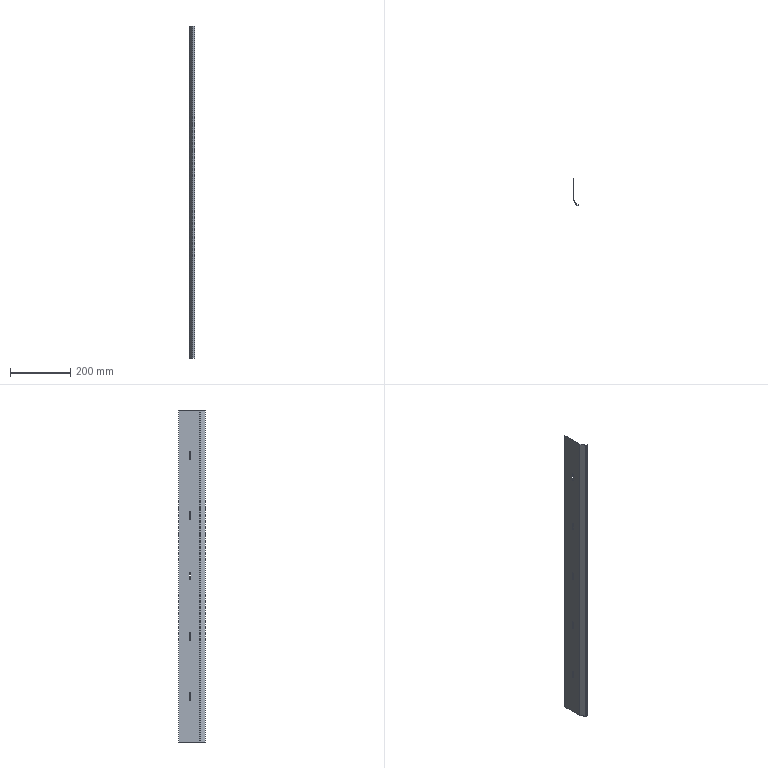Part | 1 solid | 47 faces | box 17 x 88.321 x 1100 mm | volume 105591 mm3 | plane 28 | cylinder 19 | commonest cylinder face diameters 6 x15 2 x2 4 x2
STEP:
#1=CARTESIAN_POINT('',(0.,-34.5,210.));
#2=VERTEX_POINT('',#1);
#3=CARTESIAN_POINT('',(0.,-37.5,213.));
#4=VERTEX_POINT('',#3);
#5=CARTESIAN_POINT('',(0.,-37.5,210.));
#6=DIRECTION('',(1.,0.,0.));
#7=DIRECTION('',(0.,1.,0.));
#8=AXIS2_PLACEMENT_3D('',#5,#6,#7);
#9=CIRCLE('',#8,3.);
#10=EDGE_CURVE('',#2,#4,#9,.T.);
#11=ORIENTED_EDGE('',*,*,#10,.T.);
#12=CARTESIAN_POINT('',(-1.,-37.5,213.));
#13=VERTEX_POINT('',#12);
#14=CARTESIAN_POINT('',(9.,-37.5,213.));
#15=DIRECTION('',(-1.,0.,0.));
#16=VECTOR('',#15,1000.);
#17=LINE('',#14,#16);
#18=EDGE_CURVE('',#4,#13,#17,.T.);
#19=ORIENTED_EDGE('',*,*,#18,.T.);
#20=CARTESIAN_POINT('',(-1.,-34.5,210.));
#21=VERTEX_POINT('',#20);
#22=CARTESIAN_POINT('',(-1.,-37.5,210.));
#23=DIRECTION('',(-1.,0.,0.));
#24=DIRECTION('',(0.,0.,-1.));
#25=AXIS2_PLACEMENT_3D('',#22,#23,#24);
#26=CIRCLE('',#25,3.);
#27=EDGE_CURVE('',#13,#21,#26,.T.);
#28=ORIENTED_EDGE('',*,*,#27,.T.);
#29=CARTESIAN_POINT('',(9.,-34.5,210.));
#30=DIRECTION('',(-1.,0.,0.));
#31=VECTOR('',#30,1000.);
#32=LINE('',#29,#31);
#33=EDGE_CURVE('',#2,#21,#32,.T.);
#34=ORIENTED_EDGE('',*,*,#33,.F.);
#35=EDGE_LOOP('',(#11,#19,#28,#34));
#36=FACE_OUTER_BOUND('',#35,.T.);
#37=CARTESIAN_POINT('',(9.,-37.5,210.));
#38=DIRECTION('',(-1.,0.,0.));
#39=DIRECTION('',(0.,0.,1.));
#40=AXIS2_PLACEMENT_3D('',#37,#38,#39);
#41=CYLINDRICAL_SURFACE('',#40,3.);
#42=ADVANCED_FACE('',(#36),#41,.F.);
#43=CARTESIAN_POINT('',(0.,-34.5,410.));
#44=VERTEX_POINT('',#43);
#45=CARTESIAN_POINT('',(0.,-37.5,413.));
#46=VERTEX_POINT('',#45);
#47=CARTESIAN_POINT('',(0.,-37.5,410.));
#48=DIRECTION('',(1.,0.,0.));
#49=DIRECTION('',(0.,1.,0.));
#50=AXIS2_PLACEMENT_3D('',#47,#48,#49);
#51=CIRCLE('',#50,3.);
#52=EDGE_CURVE('',#44,#46,#51,.T.);
#53=ORIENTED_EDGE('',*,*,#52,.T.);
#54=CARTESIAN_POINT('',(-1.,-37.5,413.));
#55=VERTEX_POINT('',#54);
#56=CARTESIAN_POINT('',(9.,-37.5,413.));
#57=DIRECTION('',(-1.,0.,0.));
#58=VECTOR('',#57,1000.);
#59=LINE('',#56,#58);
#60=EDGE_CURVE('',#46,#55,#59,.T.);
#61=ORIENTED_EDGE('',*,*,#60,.T.);
#62=CARTESIAN_POINT('',(-1.,-34.5,410.));
#63=VERTEX_POINT('',#62);
#64=CARTESIAN_POINT('',(-1.,-37.5,410.));
#65=DIRECTION('',(-1.,0.,0.));
#66=DIRECTION('',(0.,0.,-1.));
#67=AXIS2_PLACEMENT_3D('',#64,#65,#66);
#68=CIRCLE('',#67,3.);
#69=EDGE_CURVE('',#55,#63,#68,.T.);
#70=ORIENTED_EDGE('',*,*,#69,.T.);
#71=CARTESIAN_POINT('',(9.,-34.5,410.));
#72=DIRECTION('',(-1.,0.,0.));
#73=VECTOR('',#72,1000.);
#74=LINE('',#71,#73);
#75=EDGE_CURVE('',#44,#63,#74,.T.);
#76=ORIENTED_EDGE('',*,*,#75,.F.);
#77=EDGE_LOOP('',(#53,#61,#70,#76));
#78=FACE_OUTER_BOUND('',#77,.T.);
#79=CARTESIAN_POINT('',(9.,-37.5,410.));
#80=DIRECTION('',(-1.,0.,0.));
#81=DIRECTION('',(0.,0.,1.));
#82=AXIS2_PLACEMENT_3D('',#79,#80,#81);
#83=CYLINDRICAL_SURFACE('',#82,3.);
#84=ADVANCED_FACE('',(#78),#83,.F.);
#85=CARTESIAN_POINT('',(0.,-34.5,-390.));
#86=VERTEX_POINT('',#85);
#87=CARTESIAN_POINT('',(0.,-37.5,-387.));
#88=VERTEX_POINT('',#87);
#89=CARTESIAN_POINT('',(0.,-37.5,-390.));
#90=DIRECTION('',(1.,0.,0.));
#91=DIRECTION('',(0.,1.,0.));
#92=AXIS2_PLACEMENT_3D('',#89,#90,#91);
#93=CIRCLE('',#92,3.);
#94=EDGE_CURVE('',#86,#88,#93,.T.);
#95=ORIENTED_EDGE('',*,*,#94,.T.);
#96=CARTESIAN_POINT('',(-1.,-37.5,-387.));
#97=VERTEX_POINT('',#96);
#98=CARTESIAN_POINT('',(9.,-37.5,-387.));
#99=DIRECTION('',(-1.,0.,0.));
#100=VECTOR('',#99,1000.);
#101=LINE('',#98,#100);
#102=EDGE_CURVE('',#88,#97,#101,.T.);
#103=ORIENTED_EDGE('',*,*,#102,.T.);
#104=CARTESIAN_POINT('',(-1.,-34.5,-390.));
#105=VERTEX_POINT('',#104);
#106=CARTESIAN_POINT('',(-1.,-37.5,-390.));
#107=DIRECTION('',(-1.,0.,0.));
#108=DIRECTION('',(0.,0.,1.));
#109=AXIS2_PLACEMENT_3D('',#106,#107,#108);
#110=CIRCLE('',#109,3.);
#111=EDGE_CURVE('',#97,#105,#110,.T.);
#112=ORIENTED_EDGE('',*,*,#111,.T.);
#113=CARTESIAN_POINT('',(9.,-34.5,-390.));
#114=DIRECTION('',(-1.,0.,0.));
#115=VECTOR('',#114,1000.);
#116=LINE('',#113,#115);
#117=EDGE_CURVE('',#86,#105,#116,.T.);
#118=ORIENTED_EDGE('',*,*,#117,.F.);
#119=EDGE_LOOP('',(#95,#103,#112,#118));
#120=FACE_OUTER_BOUND('',#119,.T.);
#121=CARTESIAN_POINT('',(9.,-37.5,-390.));
#122=DIRECTION('',(-1.,0.,0.));
#123=DIRECTION('',(0.,0.,1.));
#124=AXIS2_PLACEMENT_3D('',#121,#122,#123);
#125=CYLINDRICAL_SURFACE('',#124,3.);
#126=ADVANCED_FACE('',(#120),#125,.F.);
#127=CARTESIAN_POINT('',(0.,-34.5,-190.));
#128=VERTEX_POINT('',#127);
#129=CARTESIAN_POINT('',(0.,-37.5,-187.));
#130=VERTEX_POINT('',#129);
#131=CARTESIAN_POINT('',(0.,-37.5,-190.));
#132=DIRECTION('',(1.,0.,0.));
#133=DIRECTION('',(0.,1.,0.));
#134=AXIS2_PLACEMENT_3D('',#131,#132,#133);
#135=CIRCLE('',#134,3.);
#136=EDGE_CURVE('',#128,#130,#135,.T.);
#137=ORIENTED_EDGE('',*,*,#136,.T.);
#138=CARTESIAN_POINT('',(-1.,-37.5,-187.));
#139=VERTEX_POINT('',#138);
#140=CARTESIAN_POINT('',(9.,-37.5,-187.));
#141=DIRECTION('',(-1.,0.,0.));
#142=VECTOR('',#141,1000.);
#143=LINE('',#140,#142);
#144=EDGE_CURVE('',#130,#139,#143,.T.);
#145=ORIENTED_EDGE('',*,*,#144,.T.);
#146=CARTESIAN_POINT('',(-1.,-34.5,-190.));
#147=VERTEX_POINT('',#146);
#148=CARTESIAN_POINT('',(-1.,-37.5,-190.));
#149=DIRECTION('',(-1.,0.,0.));
#150=DIRECTION('',(0.,0.,1.));
#151=AXIS2_PLACEMENT_3D('',#148,#149,#150);
#152=CIRCLE('',#151,3.);
#153=EDGE_CURVE('',#139,#147,#152,.T.);
#154=ORIENTED_EDGE('',*,*,#153,.T.);
#155=CARTESIAN_POINT('',(9.,-34.5,-190.));
#156=DIRECTION('',(-1.,0.,0.));
#157=VECTOR('',#156,1000.);
#158=LINE('',#155,#157);
#159=EDGE_CURVE('',#128,#147,#158,.T.);
#160=ORIENTED_EDGE('',*,*,#159,.F.);
#161=EDGE_LOOP('',(#137,#145,#154,#160));
#162=FACE_OUTER_BOUND('',#161,.T.);
#163=CARTESIAN_POINT('',(9.,-37.5,-190.));
#164=DIRECTION('',(-1.,0.,0.));
#165=DIRECTION('',(0.,0.,1.));
#166=AXIS2_PLACEMENT_3D('',#163,#164,#165);
#167=CYLINDRICAL_SURFACE('',#166,3.);
#168=ADVANCED_FACE('',(#162),#167,.F.);
#169=CARTESIAN_POINT('',(0.,-34.5,10.));
#170=VERTEX_POINT('',#169);
#171=CARTESIAN_POINT('',(0.,-37.5,13.));
#172=VERTEX_POINT('',#171);
#173=CARTESIAN_POINT('',(0.,-37.5,10.));
#174=DIRECTION('',(1.,0.,0.));
#175=DIRECTION('',(0.,1.,0.));
#176=AXIS2_PLACEMENT_3D('',#173,#174,#175);
#177=CIRCLE('',#176,3.);
#178=EDGE_CURVE('',#170,#172,#177,.T.);
#179=ORIENTED_EDGE('',*,*,#178,.T.);
#180=CARTESIAN_POINT('',(-1.,-37.5,13.));
#181=VERTEX_POINT('',#180);
#182=CARTESIAN_POINT('',(9.,-37.5,13.));
#183=DIRECTION('',(-1.,0.,0.));
#184=VECTOR('',#183,1000.);
#185=LINE('',#182,#184);
#186=EDGE_CURVE('',#172,#181,#185,.T.);
#187=ORIENTED_EDGE('',*,*,#186,.T.);
#188=CARTESIAN_POINT('',(-1.,-34.5,10.));
#189=VERTEX_POINT('',#188);
#190=CARTESIAN_POINT('',(-1.,-37.5,10.));
#191=DIRECTION('',(-1.,0.,0.));
#192=DIRECTION('',(0.,0.,1.));
#193=AXIS2_PLACEMENT_3D('',#190,#191,#192);
#194=CIRCLE('',#193,3.);
#195=EDGE_CURVE('',#181,#189,#194,.T.);
#196=ORIENTED_EDGE('',*,*,#195,.T.);
#197=CARTESIAN_POINT('',(9.,-34.5,10.));
#198=DIRECTION('',(-1.,0.,0.));
#199=VECTOR('',#198,1000.);
#200=LINE('',#197,#199);
#201=EDGE_CURVE('',#170,#189,#200,.T.);
#202=ORIENTED_EDGE('',*,*,#201,.F.);
#203=EDGE_LOOP('',(#179,#187,#196,#202));
#204=FACE_OUTER_BOUND('',#203,.T.);
#205=CARTESIAN_POINT('',(9.,-37.5,10.));
#206=DIRECTION('',(-1.,0.,0.));
#207=DIRECTION('',(0.,0.,1.));
#208=AXIS2_PLACEMENT_3D('',#205,#206,#207);
#209=CYLINDRICAL_SURFACE('',#208,3.);
#210=ADVANCED_FACE('',(#204),#209,.F.);
#211=CARTESIAN_POINT('',(0.134,-70.232,550.));
#212=VERTEX_POINT('',#211);
#213=CARTESIAN_POINT('',(-0.7321,-70.732,550.));
#214=VERTEX_POINT('',#213);
#215=CARTESIAN_POINT('',(0.134,-70.232,550.));
#216=DIRECTION('',(-0.866,-0.5,0.));
#217=VECTOR('',#216,1000.);
#218=LINE('',#215,#217);
#219=EDGE_CURVE('',#212,#214,#218,.T.);
#220=ORIENTED_EDGE('',*,*,#219,.F.);
#221=CARTESIAN_POINT('',(0.,-69.732,550.));
#222=VERTEX_POINT('',#221);
#223=CARTESIAN_POINT('',(1.,-69.732,550.));
#224=DIRECTION('',(0.,0.,1.));
#225=DIRECTION('',(-1.,0.,0.));
#226=AXIS2_PLACEMENT_3D('',#223,#224,#225);
#227=CIRCLE('',#226,1.);
#228=EDGE_CURVE('',#222,#212,#227,.T.);
#229=ORIENTED_EDGE('',*,*,#228,.F.);
#230=CARTESIAN_POINT('',(-1.,-69.732,550.));
#231=VERTEX_POINT('',#230);
#232=CARTESIAN_POINT('',(-1.,-69.732,550.));
#233=DIRECTION('',(1.,0.,0.));
#234=VECTOR('',#233,1000.);
#235=LINE('',#232,#234);
#236=EDGE_CURVE('',#231,#222,#235,.T.);
#237=ORIENTED_EDGE('',*,*,#236,.F.);
#238=CARTESIAN_POINT('',(1.,-69.732,550.));
#239=DIRECTION('',(0.,0.,1.));
#240=DIRECTION('',(1.,0.,0.));
#241=AXIS2_PLACEMENT_3D('',#238,#239,#240);
#242=CIRCLE('',#241,2.);
#243=EDGE_CURVE('',#231,#214,#242,.T.);
#244=ORIENTED_EDGE('',*,*,#243,.T.);
#245=EDGE_LOOP('',(#220,#229,#237,#244));
#246=FACE_OUTER_BOUND('',#245,.T.);
#247=CARTESIAN_POINT('',(0.134,-70.232,550.));
#248=DIRECTION('',(0.,0.,1.));
#249=DIRECTION('',(1.,0.,0.));
#250=AXIS2_PLACEMENT_3D('',#247,#248,#249);
#251=PLANE('',#250);
#252=ADVANCED_FACE('',(#246),#251,.T.);
#253=CARTESIAN_POINT('',(9.711,-86.821,550.));
#254=VERTEX_POINT('',#253);
#255=CARTESIAN_POINT('',(0.,-70.,550.));
#256=DIRECTION('',(0.5,-0.866,0.));
#257=VECTOR('',#256,1000.);
#258=LINE('',#255,#257);
#259=EDGE_CURVE('',#212,#254,#258,.T.);
#260=ORIENTED_EDGE('',*,*,#259,.F.);
#261=ORIENTED_EDGE('',*,*,#219,.T.);
#262=CARTESIAN_POINT('',(8.845,-87.321,550.));
#263=VERTEX_POINT('',#262);
#264=CARTESIAN_POINT('',(-0.866,-70.5,550.));
#265=DIRECTION('',(0.5,-0.866,0.));
#266=VECTOR('',#265,1000.);
#267=LINE('',#264,#266);
#268=EDGE_CURVE('',#214,#263,#267,.T.);
#269=ORIENTED_EDGE('',*,*,#268,.T.);
#270=CARTESIAN_POINT('',(8.845,-87.321,550.));
#271=DIRECTION('',(0.866,0.5,0.));
#272=VECTOR('',#271,1000.);
#273=LINE('',#270,#272);
#274=EDGE_CURVE('',#263,#254,#273,.T.);
#275=ORIENTED_EDGE('',*,*,#274,.T.);
#276=EDGE_LOOP('',(#260,#261,#269,#275));
#277=FACE_OUTER_BOUND('',#276,.T.);
#278=CARTESIAN_POINT('',(-1.,-69.732,550.));
#279=DIRECTION('',(0.,0.,1.));
#280=DIRECTION('',(1.,0.,0.));
#281=AXIS2_PLACEMENT_3D('',#278,#279,#280);
#282=PLANE('',#281);
#283=ADVANCED_FACE('',(#277),#282,.T.);
#284=CARTESIAN_POINT('',(0.,-69.732,-550.));
#285=VERTEX_POINT('',#284);
#286=CARTESIAN_POINT('',(-1.,-69.732,-550.));
#287=VERTEX_POINT('',#286);
#288=CARTESIAN_POINT('',(0.,-69.732,-550.));
#289=DIRECTION('',(-1.,0.,0.));
#290=VECTOR('',#289,1000.);
#291=LINE('',#288,#290);
#292=EDGE_CURVE('',#285,#287,#291,.T.);
#293=ORIENTED_EDGE('',*,*,#292,.F.);
#294=CARTESIAN_POINT('',(0.134,-70.232,-550.));
#295=VERTEX_POINT('',#294);
#296=CARTESIAN_POINT('',(1.,-69.732,-550.));
#297=DIRECTION('',(0.,0.,1.));
#298=DIRECTION('',(-1.,0.,0.));
#299=AXIS2_PLACEMENT_3D('',#296,#297,#298);
#300=CIRCLE('',#299,1.);
#301=EDGE_CURVE('',#285,#295,#300,.T.);
#302=ORIENTED_EDGE('',*,*,#301,.T.);
#303=CARTESIAN_POINT('',(-0.7321,-70.732,-550.));
#304=VERTEX_POINT('',#303);
#305=CARTESIAN_POINT('',(-0.7321,-70.732,-550.));
#306=DIRECTION('',(0.866,0.5,0.));
#307=VECTOR('',#306,1000.);
#308=LINE('',#305,#307);
#309=EDGE_CURVE('',#304,#295,#308,.T.);
#310=ORIENTED_EDGE('',*,*,#309,.F.);
#311=CARTESIAN_POINT('',(1.,-69.732,-550.));
#312=DIRECTION('',(0.,0.,1.));
#313=DIRECTION('',(1.,0.,0.));
#314=AXIS2_PLACEMENT_3D('',#311,#312,#313);
#315=CIRCLE('',#314,2.);
#316=EDGE_CURVE('',#287,#304,#315,.T.);
#317=ORIENTED_EDGE('',*,*,#316,.F.);
#318=EDGE_LOOP('',(#293,#302,#310,#317));
#319=FACE_OUTER_BOUND('',#318,.T.);
#320=CARTESIAN_POINT('',(0.,-69.732,-550.));
#321=DIRECTION('',(0.,0.,-1.));
#322=DIRECTION('',(-1.,0.,0.));
#323=AXIS2_PLACEMENT_3D('',#320,#321,#322);
#324=PLANE('',#323);
#325=ADVANCED_FACE('',(#319),#324,.T.);
#326=CARTESIAN_POINT('',(0.,0.,-550.));
#327=VERTEX_POINT('',#326);
#328=CARTESIAN_POINT('',(0.,0.,-550.));
#329=DIRECTION('',(0.,-1.,0.));
#330=VECTOR('',#329,1000.);
#331=LINE('',#328,#330);
#332=EDGE_CURVE('',#327,#285,#331,.T.);
#333=ORIENTED_EDGE('',*,*,#332,.T.);
#334=ORIENTED_EDGE('',*,*,#292,.T.);
#335=CARTESIAN_POINT('',(-1.,0.,-550.));
#336=VERTEX_POINT('',#335);
#337=CARTESIAN_POINT('',(-1.,0.,-550.));
#338=DIRECTION('',(0.,-1.,0.));
#339=VECTOR('',#338,1000.);
#340=LINE('',#337,#339);
#341=EDGE_CURVE('',#336,#287,#340,.T.);
#342=ORIENTED_EDGE('',*,*,#341,.F.);
#343=CARTESIAN_POINT('',(-1.,0.,-550.));
#344=DIRECTION('',(1.,0.,0.));
#345=VECTOR('',#344,1000.);
#346=LINE('',#343,#345);
#347=EDGE_CURVE('',#336,#327,#346,.T.);
#348=ORIENTED_EDGE('',*,*,#347,.T.);
#349=EDGE_LOOP('',(#333,#334,#342,#348));
#350=FACE_OUTER_BOUND('',#349,.T.);
#351=CARTESIAN_POINT('',(-0.7321,-70.732,-550.));
#352=DIRECTION('',(0.,0.,-1.));
#353=DIRECTION('',(-1.,0.,0.));
#354=AXIS2_PLACEMENT_3D('',#351,#352,#353);
#355=PLANE('',#354);
#356=ADVANCED_FACE('',(#350),#355,.T.);
#357=CARTESIAN_POINT('',(10.577,-87.321,550.));
#358=VERTEX_POINT('',#357);
#359=CARTESIAN_POINT('',(10.577,-88.321,550.));
#360=VERTEX_POINT('',#359);
#361=CARTESIAN_POINT('',(10.577,-87.321,550.));
#362=DIRECTION('',(0.,-1.,0.));
#363=VECTOR('',#362,1000.);
#364=LINE('',#361,#363);
#365=EDGE_CURVE('',#358,#360,#364,.T.);
#366=ORIENTED_EDGE('',*,*,#365,.F.);
#367=CARTESIAN_POINT('',(10.577,-86.321,550.));
#368=DIRECTION('',(0.,0.,1.));
#369=DIRECTION('',(-1.,0.,0.));
#370=AXIS2_PLACEMENT_3D('',#367,#368,#369);
#371=CIRCLE('',#370,1.);
#372=EDGE_CURVE('',#254,#358,#371,.T.);
#373=ORIENTED_EDGE('',*,*,#372,.F.);
#374=ORIENTED_EDGE('',*,*,#274,.F.);
#375=CARTESIAN_POINT('',(10.577,-86.321,550.));
#376=DIRECTION('',(0.,0.,1.));
#377=DIRECTION('',(1.,0.,0.));
#378=AXIS2_PLACEMENT_3D('',#375,#376,#377);
#379=CIRCLE('',#378,2.);
#380=EDGE_CURVE('',#263,#360,#379,.T.);
#381=ORIENTED_EDGE('',*,*,#380,.T.);
#382=EDGE_LOOP('',(#366,#373,#374,#381));
#383=FACE_OUTER_BOUND('',#382,.T.);
#384=CARTESIAN_POINT('',(10.577,-87.321,550.));
#385=DIRECTION('',(0.,0.,1.));
#386=DIRECTION('',(1.,0.,0.));
#387=AXIS2_PLACEMENT_3D('',#384,#385,#386);
#388=PLANE('',#387);
#389=ADVANCED_FACE('',(#383),#388,.T.);
#390=CARTESIAN_POINT('',(16.,-87.321,550.));
#391=VERTEX_POINT('',#390);
#392=CARTESIAN_POINT('',(10.,-87.321,550.));
#393=DIRECTION('',(1.,0.,0.));
#394=VECTOR('',#393,1000.);
#395=LINE('',#392,#394);
#396=EDGE_CURVE('',#358,#391,#395,.T.);
#397=ORIENTED_EDGE('',*,*,#396,.F.);
#398=ORIENTED_EDGE('',*,*,#365,.T.);
#399=CARTESIAN_POINT('',(16.,-88.321,550.));
#400=VERTEX_POINT('',#399);
#401=CARTESIAN_POINT('',(10.,-88.321,550.));
#402=DIRECTION('',(1.,0.,0.));
#403=VECTOR('',#402,1000.);
#404=LINE('',#401,#403);
#405=EDGE_CURVE('',#360,#400,#404,.T.);
#406=ORIENTED_EDGE('',*,*,#405,.T.);
#407=CARTESIAN_POINT('',(16.,-87.321,550.));
#408=DIRECTION('',(0.,-1.,0.));
#409=VECTOR('',#408,1000.);
#410=LINE('',#407,#409);
#411=EDGE_CURVE('',#391,#400,#410,.T.);
#412=ORIENTED_EDGE('',*,*,#411,.F.);
#413=EDGE_LOOP('',(#397,#398,#406,#412));
#414=FACE_OUTER_BOUND('',#413,.T.);
#415=CARTESIAN_POINT('',(8.845,-87.321,550.));
#416=DIRECTION('',(0.,0.,1.));
#417=DIRECTION('',(1.,0.,0.));
#418=AXIS2_PLACEMENT_3D('',#415,#416,#417);
#419=PLANE('',#418);
#420=ADVANCED_FACE('',(#414),#419,.T.);
#421=CARTESIAN_POINT('',(9.711,-86.821,-550.));
#422=VERTEX_POINT('',#421);
#423=CARTESIAN_POINT('',(8.845,-87.321,-550.));
#424=VERTEX_POINT('',#423);
#425=CARTESIAN_POINT('',(9.711,-86.821,-550.));
#426=DIRECTION('',(-0.866,-0.5,0.));
#427=VECTOR('',#426,1000.);
#428=LINE('',#425,#427);
#429=EDGE_CURVE('',#422,#424,#428,.T.);
#430=ORIENTED_EDGE('',*,*,#429,.F.);
#431=CARTESIAN_POINT('',(10.577,-87.321,-550.));
#432=VERTEX_POINT('',#431);
#433=CARTESIAN_POINT('',(10.577,-86.321,-550.));
#434=DIRECTION('',(0.,0.,1.));
#435=DIRECTION('',(-1.,0.,0.));
#436=AXIS2_PLACEMENT_3D('',#433,#434,#435);
#437=CIRCLE('',#436,1.);
#438=EDGE_CURVE('',#422,#432,#437,.T.);
#439=ORIENTED_EDGE('',*,*,#438,.T.);
#440=CARTESIAN_POINT('',(10.577,-88.321,-550.));
#441=VERTEX_POINT('',#440);
#442=CARTESIAN_POINT('',(10.577,-88.321,-550.));
#443=DIRECTION('',(0.,1.,0.));
#444=VECTOR('',#443,1000.);
#445=LINE('',#442,#444);
#446=EDGE_CURVE('',#441,#432,#445,.T.);
#447=ORIENTED_EDGE('',*,*,#446,.F.);
#448=CARTESIAN_POINT('',(10.577,-86.321,-550.));
#449=DIRECTION('',(0.,0.,1.));
#450=DIRECTION('',(1.,0.,0.));
#451=AXIS2_PLACEMENT_3D('',#448,#449,#450);
#452=CIRCLE('',#451,2.);
#453=EDGE_CURVE('',#424,#441,#452,.T.);
#454=ORIENTED_EDGE('',*,*,#453,.F.);
#455=EDGE_LOOP('',(#430,#439,#447,#454));
#456=FACE_OUTER_BOUND('',#455,.T.);
#457=CARTESIAN_POINT('',(9.711,-86.821,-550.));
#458=DIRECTION('',(0.,0.,-1.));
#459=DIRECTION('',(-1.,0.,0.));
#460=AXIS2_PLACEMENT_3D('',#457,#458,#459);
#461=PLANE('',#460);
#462=ADVANCED_FACE('',(#456),#461,.T.);
#463=CARTESIAN_POINT('',(0.,-70.,-550.));
#464=DIRECTION('',(0.5,-0.866,0.));
#465=VECTOR('',#464,1000.);
#466=LINE('',#463,#465);
#467=EDGE_CURVE('',#295,#422,#466,.T.);
#468=ORIENTED_EDGE('',*,*,#467,.T.);
#469=ORIENTED_EDGE('',*,*,#429,.T.);
#470=CARTESIAN_POINT('',(-0.866,-70.5,-550.));
#471=DIRECTION('',(0.5,-0.866,0.));
#472=VECTOR('',#471,1000.);
#473=LINE('',#470,#472);
#474=EDGE_CURVE('',#304,#424,#473,.T.);
#475=ORIENTED_EDGE('',*,*,#474,.F.);
#476=ORIENTED_EDGE('',*,*,#309,.T.);
#477=EDGE_LOOP('',(#468,#469,#475,#476));
#478=FACE_OUTER_BOUND('',#477,.T.);
#479=CARTESIAN_POINT('',(10.577,-88.321,-550.));
#480=DIRECTION('',(0.,0.,-1.));
#481=DIRECTION('',(-1.,0.,0.));
#482=AXIS2_PLACEMENT_3D('',#479,#480,#481);
#483=PLANE('',#482);
#484=ADVANCED_FACE('',(#478),#483,.T.);
#485=CARTESIAN_POINT('',(16.,-88.321,-550.));
#486=VERTEX_POINT('',#485);
#487=CARTESIAN_POINT('',(10.,-88.321,-550.));
#488=DIRECTION('',(1.,0.,0.));
#489=VECTOR('',#488,1000.);
#490=LINE('',#487,#489);
#491=EDGE_CURVE('',#441,#486,#490,.T.);
#492=ORIENTED_EDGE('',*,*,#491,.T.);
#493=CARTESIAN_POINT('',(16.,-88.321,550.));
#494=DIRECTION('',(0.,0.,-1.));
#495=VECTOR('',#494,1000.);
#496=LINE('',#493,#495);
#497=EDGE_CURVE('',#400,#486,#496,.T.);
#498=ORIENTED_EDGE('',*,*,#497,.F.);
#499=ORIENTED_EDGE('',*,*,#405,.F.);
#500=CARTESIAN_POINT('',(10.577,-88.321,550.));
#501=DIRECTION('',(0.,0.,-1.));
#502=VECTOR('',#501,1000.);
#503=LINE('',#500,#502);
#504=EDGE_CURVE('',#360,#441,#503,.T.);
#505=ORIENTED_EDGE('',*,*,#504,.T.);
#506=EDGE_LOOP('',(#492,#498,#499,#505));
#507=FACE_OUTER_BOUND('',#506,.T.);
#508=CARTESIAN_POINT('',(10.,-88.321,550.));
#509=DIRECTION('',(0.,1.,0.));
#510=DIRECTION('',(-1.,0.,0.));
#511=AXIS2_PLACEMENT_3D('',#508,#509,#510);
#512=PLANE('',#511);
#513=ADVANCED_FACE('',(#507),#512,.F.);
#514=CARTESIAN_POINT('',(16.,-87.321,-550.));
#515=VERTEX_POINT('',#514);
#516=CARTESIAN_POINT('',(16.,-87.321,-550.));
#517=DIRECTION('',(0.,-1.,0.));
#518=VECTOR('',#517,1000.);
#519=LINE('',#516,#518);
#520=EDGE_CURVE('',#515,#486,#519,.T.);
#521=ORIENTED_EDGE('',*,*,#520,.F.);
#522=CARTESIAN_POINT('',(16.,-87.321,550.));
#523=DIRECTION('',(0.,0.,-1.));
#524=VECTOR('',#523,1000.);
#525=LINE('',#522,#524);
#526=EDGE_CURVE('',#391,#515,#525,.T.);
#527=ORIENTED_EDGE('',*,*,#526,.F.);
#528=ORIENTED_EDGE('',*,*,#411,.T.);
#529=ORIENTED_EDGE('',*,*,#497,.T.);
#530=EDGE_LOOP('',(#521,#527,#528,#529));
#531=FACE_OUTER_BOUND('',#530,.T.);
#532=CARTESIAN_POINT('',(16.,-87.321,550.));
#533=DIRECTION('',(1.,0.,0.));
#534=DIRECTION('',(0.,1.,0.));
#535=AXIS2_PLACEMENT_3D('',#532,#533,#534);
#536=PLANE('',#535);
#537=ADVANCED_FACE('',(#531),#536,.T.);
#538=CARTESIAN_POINT('',(10.,-87.321,-550.));
#539=DIRECTION('',(1.,0.,0.));
#540=VECTOR('',#539,1000.);
#541=LINE('',#538,#540);
#542=EDGE_CURVE('',#432,#515,#541,.T.);
#543=ORIENTED_EDGE('',*,*,#542,.F.);
#544=CARTESIAN_POINT('',(10.577,-87.321,550.));
#545=DIRECTION('',(0.,0.,-1.));
#546=VECTOR('',#545,1000.);
#547=LINE('',#544,#546);
#548=EDGE_CURVE('',#358,#432,#547,.T.);
#549=ORIENTED_EDGE('',*,*,#548,.F.);
#550=ORIENTED_EDGE('',*,*,#396,.T.);
#551=ORIENTED_EDGE('',*,*,#526,.T.);
#552=EDGE_LOOP('',(#543,#549,#550,#551));
#553=FACE_OUTER_BOUND('',#552,.T.);
#554=CARTESIAN_POINT('',(10.,-87.321,550.));
#555=DIRECTION('',(0.,1.,0.));
#556=DIRECTION('',(-1.,0.,0.));
#557=AXIS2_PLACEMENT_3D('',#554,#555,#556);
#558=PLANE('',#557);
#559=ADVANCED_FACE('',(#553),#558,.T.);
#560=ORIENTED_EDGE('',*,*,#438,.F.);
#561=CARTESIAN_POINT('',(9.711,-86.821,550.));
#562=DIRECTION('',(0.,0.,-1.));
#563=VECTOR('',#562,1000.);
#564=LINE('',#561,#563);
#565=EDGE_CURVE('',#254,#422,#564,.T.);
#566=ORIENTED_EDGE('',*,*,#565,.F.);
#567=ORIENTED_EDGE('',*,*,#372,.T.);
#568=ORIENTED_EDGE('',*,*,#548,.T.);
#569=EDGE_LOOP('',(#560,#566,#567,#568));
#570=FACE_OUTER_BOUND('',#569,.T.);
#571=CARTESIAN_POINT('',(10.577,-86.321,550.));
#572=DIRECTION('',(0.,0.,-1.));
#573=DIRECTION('',(-1.,0.,0.));
#574=AXIS2_PLACEMENT_3D('',#571,#572,#573);
#575=CYLINDRICAL_SURFACE('',#574,1.);
#576=ADVANCED_FACE('',(#570),#575,.F.);
#577=ORIENTED_EDGE('',*,*,#467,.F.);
#578=CARTESIAN_POINT('',(0.134,-70.232,550.));
#579=DIRECTION('',(0.,0.,-1.));
#580=VECTOR('',#579,1000.);
#581=LINE('',#578,#580);
#582=EDGE_CURVE('',#212,#295,#581,.T.);
#583=ORIENTED_EDGE('',*,*,#582,.F.);
#584=ORIENTED_EDGE('',*,*,#259,.T.);
#585=ORIENTED_EDGE('',*,*,#565,.T.);
#586=EDGE_LOOP('',(#577,#583,#584,#585));
#587=FACE_OUTER_BOUND('',#586,.T.);
#588=CARTESIAN_POINT('',(0.,-70.,550.));
#589=DIRECTION('',(0.866,0.5,0.));
#590=DIRECTION('',(-0.5,0.866,0.));
#591=AXIS2_PLACEMENT_3D('',#588,#589,#590);
#592=PLANE('',#591);
#593=ADVANCED_FACE('',(#587),#592,.T.);
#594=ORIENTED_EDGE('',*,*,#301,.F.);
#595=CARTESIAN_POINT('',(0.,-69.732,550.));
#596=DIRECTION('',(0.,0.,-1.));
#597=VECTOR('',#596,1000.);
#598=LINE('',#595,#597);
#599=EDGE_CURVE('',#222,#285,#598,.T.);
#600=ORIENTED_EDGE('',*,*,#599,.F.);
#601=ORIENTED_EDGE('',*,*,#228,.T.);
#602=ORIENTED_EDGE('',*,*,#582,.T.);
#603=EDGE_LOOP('',(#594,#600,#601,#602));
#604=FACE_OUTER_BOUND('',#603,.T.);
#605=CARTESIAN_POINT('',(1.,-69.732,550.));
#606=DIRECTION('',(0.,0.,-1.));
#607=DIRECTION('',(-1.,0.,0.));
#608=AXIS2_PLACEMENT_3D('',#605,#606,#607);
#609=CYLINDRICAL_SURFACE('',#608,1.);
#610=ADVANCED_FACE('',(#604),#609,.F.);
#611=ORIENTED_EDGE('',*,*,#10,.F.);
#612=CARTESIAN_POINT('',(0.,-34.5,190.));
#613=VERTEX_POINT('',#612);
#614=CARTESIAN_POINT('',(0.,-34.5,550.));
#615=DIRECTION('',(0.,0.,1.));
#616=VECTOR('',#615,1000.);
#617=LINE('',#614,#616);
#618=EDGE_CURVE('',#613,#2,#617,.T.);
#619=ORIENTED_EDGE('',*,*,#618,.F.);
#620=CARTESIAN_POINT('',(0.,-40.5,190.));
#621=VERTEX_POINT('',#620);
#622=CARTESIAN_POINT('',(0.,-37.5,190.));
#623=DIRECTION('',(1.,0.,0.));
#624=DIRECTION('',(0.,1.,0.));
#625=AXIS2_PLACEMENT_3D('',#622,#623,#624);
#626=CIRCLE('',#625,3.);
#627=EDGE_CURVE('',#621,#613,#626,.T.);
#628=ORIENTED_EDGE('',*,*,#627,.F.);
#629=CARTESIAN_POINT('',(0.,-40.5,210.));
#630=VERTEX_POINT('',#629);
#631=CARTESIAN_POINT('',(0.,-40.5,550.));
#632=DIRECTION('',(0.,0.,-1.));
#633=VECTOR('',#632,1000.);
#634=LINE('',#631,#633);
#635=EDGE_CURVE('',#630,#621,#634,.T.);
#636=ORIENTED_EDGE('',*,*,#635,.F.);
#637=CARTESIAN_POINT('',(0.,-37.5,210.));
#638=DIRECTION('',(1.,0.,0.));
#639=DIRECTION('',(0.,1.,0.));
#640=AXIS2_PLACEMENT_3D('',#637,#638,#639);
#641=CIRCLE('',#640,3.);
#642=EDGE_CURVE('',#4,#630,#641,.T.);
#643=ORIENTED_EDGE('',*,*,#642,.F.);
#644=EDGE_LOOP('',(#611,#619,#628,#636,#643));
#645=FACE_BOUND('',#644,.T.);
#646=ORIENTED_EDGE('',*,*,#52,.F.);
#647=CARTESIAN_POINT('',(0.,-34.5,390.));
#648=VERTEX_POINT('',#647);
#649=CARTESIAN_POINT('',(0.,-34.5,550.));
#650=DIRECTION('',(0.,0.,1.));
#651=VECTOR('',#650,1000.);
#652=LINE('',#649,#651);
#653=EDGE_CURVE('',#648,#44,#652,.T.);
#654=ORIENTED_EDGE('',*,*,#653,.F.);
#655=CARTESIAN_POINT('',(0.,-40.5,390.));
#656=VERTEX_POINT('',#655);
#657=CARTESIAN_POINT('',(0.,-37.5,390.));
#658=DIRECTION('',(1.,0.,0.));
#659=DIRECTION('',(0.,1.,0.));
#660=AXIS2_PLACEMENT_3D('',#657,#658,#659);
#661=CIRCLE('',#660,3.);
#662=EDGE_CURVE('',#656,#648,#661,.T.);
#663=ORIENTED_EDGE('',*,*,#662,.F.);
#664=CARTESIAN_POINT('',(0.,-40.5,410.));
#665=VERTEX_POINT('',#664);
#666=CARTESIAN_POINT('',(0.,-40.5,550.));
#667=DIRECTION('',(0.,0.,-1.));
#668=VECTOR('',#667,1000.);
#669=LINE('',#666,#668);
#670=EDGE_CURVE('',#665,#656,#669,.T.);
#671=ORIENTED_EDGE('',*,*,#670,.F.);
#672=CARTESIAN_POINT('',(0.,-37.5,410.));
#673=DIRECTION('',(1.,0.,0.));
#674=DIRECTION('',(0.,1.,0.));
#675=AXIS2_PLACEMENT_3D('',#672,#673,#674);
#676=CIRCLE('',#675,3.);
#677=EDGE_CURVE('',#46,#665,#676,.T.);
#678=ORIENTED_EDGE('',*,*,#677,.F.);
#679=EDGE_LOOP('',(#646,#654,#663,#671,#678));
#680=FACE_BOUND('',#679,.T.);
#681=CARTESIAN_POINT('',(0.,-40.5,-410.));
#682=VERTEX_POINT('',#681);
#683=CARTESIAN_POINT('',(0.,-34.5,-410.));
#684=VERTEX_POINT('',#683);
#685=CARTESIAN_POINT('',(0.,-37.5,-410.));
#686=DIRECTION('',(1.,0.,0.));
#687=DIRECTION('',(0.,1.,0.));
#688=AXIS2_PLACEMENT_3D('',#685,#686,#687);
#689=CIRCLE('',#688,3.);
#690=EDGE_CURVE('',#682,#684,#689,.T.);
#691=ORIENTED_EDGE('',*,*,#690,.F.);
#692=CARTESIAN_POINT('',(0.,-40.5,-390.));
#693=VERTEX_POINT('',#692);
#694=CARTESIAN_POINT('',(0.,-40.5,550.));
#695=DIRECTION('',(0.,0.,-1.));
#696=VECTOR('',#695,1000.);
#697=LINE('',#694,#696);
#698=EDGE_CURVE('',#693,#682,#697,.T.);
#699=ORIENTED_EDGE('',*,*,#698,.F.);
#700=CARTESIAN_POINT('',(0.,-37.5,-390.));
#701=DIRECTION('',(1.,0.,0.));
#702=DIRECTION('',(0.,1.,0.));
#703=AXIS2_PLACEMENT_3D('',#700,#701,#702);
#704=CIRCLE('',#703,3.);
#705=EDGE_CURVE('',#88,#693,#704,.T.);
#706=ORIENTED_EDGE('',*,*,#705,.F.);
#707=ORIENTED_EDGE('',*,*,#94,.F.);
#708=CARTESIAN_POINT('',(0.,-34.5,550.));
#709=DIRECTION('',(0.,0.,1.));
#710=VECTOR('',#709,1000.);
#711=LINE('',#708,#710);
#712=EDGE_CURVE('',#684,#86,#711,.T.);
#713=ORIENTED_EDGE('',*,*,#712,.F.);
#714=EDGE_LOOP('',(#691,#699,#706,#707,#713));
#715=FACE_BOUND('',#714,.T.);
#716=CARTESIAN_POINT('',(0.,-40.5,-210.));
#717=VERTEX_POINT('',#716);
#718=CARTESIAN_POINT('',(0.,-34.5,-210.));
#719=VERTEX_POINT('',#718);
#720=CARTESIAN_POINT('',(0.,-37.5,-210.));
#721=DIRECTION('',(1.,0.,0.));
#722=DIRECTION('',(0.,1.,0.));
#723=AXIS2_PLACEMENT_3D('',#720,#721,#722);
#724=CIRCLE('',#723,3.);
#725=EDGE_CURVE('',#717,#719,#724,.T.);
#726=ORIENTED_EDGE('',*,*,#725,.F.);
#727=CARTESIAN_POINT('',(0.,-40.5,-190.));
#728=VERTEX_POINT('',#727);
#729=CARTESIAN_POINT('',(0.,-40.5,550.));
#730=DIRECTION('',(0.,0.,-1.));
#731=VECTOR('',#730,1000.);
#732=LINE('',#729,#731);
#733=EDGE_CURVE('',#728,#717,#732,.T.);
#734=ORIENTED_EDGE('',*,*,#733,.F.);
#735=CARTESIAN_POINT('',(0.,-37.5,-190.));
#736=DIRECTION('',(1.,0.,0.));
#737=DIRECTION('',(0.,1.,0.));
#738=AXIS2_PLACEMENT_3D('',#735,#736,#737);
#739=CIRCLE('',#738,3.);
#740=EDGE_CURVE('',#130,#728,#739,.T.);
#741=ORIENTED_EDGE('',*,*,#740,.F.);
#742=ORIENTED_EDGE('',*,*,#136,.F.);
#743=CARTESIAN_POINT('',(0.,-34.5,550.));
#744=DIRECTION('',(0.,0.,1.));
#745=VECTOR('',#744,1000.);
#746=LINE('',#743,#745);
#747=EDGE_CURVE('',#719,#128,#746,.T.);
#748=ORIENTED_EDGE('',*,*,#747,.F.);
#749=EDGE_LOOP('',(#726,#734,#741,#742,#748));
#750=FACE_BOUND('',#749,.T.);
#751=CARTESIAN_POINT('',(0.,-40.5,-10.));
#752=VERTEX_POINT('',#751);
#753=CARTESIAN_POINT('',(0.,-34.5,-10.));
#754=VERTEX_POINT('',#753);
#755=CARTESIAN_POINT('',(0.,-37.5,-10.));
#756=DIRECTION('',(1.,0.,0.));
#757=DIRECTION('',(0.,1.,0.));
#758=AXIS2_PLACEMENT_3D('',#755,#756,#757);
#759=CIRCLE('',#758,3.);
#760=EDGE_CURVE('',#752,#754,#759,.T.);
#761=ORIENTED_EDGE('',*,*,#760,.F.);
#762=CARTESIAN_POINT('',(0.,-40.5,10.));
#763=VERTEX_POINT('',#762);
#764=CARTESIAN_POINT('',(0.,-40.5,550.));
#765=DIRECTION('',(0.,0.,-1.));
#766=VECTOR('',#765,1000.);
#767=LINE('',#764,#766);
#768=EDGE_CURVE('',#763,#752,#767,.T.);
#769=ORIENTED_EDGE('',*,*,#768,.F.);
#770=CARTESIAN_POINT('',(0.,-37.5,10.));
#771=DIRECTION('',(1.,0.,0.));
#772=DIRECTION('',(0.,1.,0.));
#773=AXIS2_PLACEMENT_3D('',#770,#771,#772);
#774=CIRCLE('',#773,3.);
#775=EDGE_CURVE('',#172,#763,#774,.T.);
#776=ORIENTED_EDGE('',*,*,#775,.F.);
#777=ORIENTED_EDGE('',*,*,#178,.F.);
#778=CARTESIAN_POINT('',(0.,-34.5,550.));
#779=DIRECTION('',(0.,0.,1.));
#780=VECTOR('',#779,1000.);
#781=LINE('',#778,#780);
#782=EDGE_CURVE('',#754,#170,#781,.T.);
#783=ORIENTED_EDGE('',*,*,#782,.F.);
#784=EDGE_LOOP('',(#761,#769,#776,#777,#783));
#785=FACE_BOUND('',#784,.T.);
#786=ORIENTED_EDGE('',*,*,#332,.F.);
#787=CARTESIAN_POINT('',(0.,0.,550.));
#788=VERTEX_POINT('',#787);
#789=CARTESIAN_POINT('',(0.,0.,550.));
#790=DIRECTION('',(0.,0.,-1.));
#791=VECTOR('',#790,1000.);
#792=LINE('',#789,#791);
#793=EDGE_CURVE('',#788,#327,#792,.T.);
#794=ORIENTED_EDGE('',*,*,#793,.F.);
#795=CARTESIAN_POINT('',(0.,0.,550.));
#796=DIRECTION('',(0.,-1.,0.));
#797=VECTOR('',#796,1000.);
#798=LINE('',#795,#797);
#799=EDGE_CURVE('',#788,#222,#798,.T.);
#800=ORIENTED_EDGE('',*,*,#799,.T.);
#801=ORIENTED_EDGE('',*,*,#599,.T.);
#802=EDGE_LOOP('',(#786,#794,#800,#801));
#803=FACE_OUTER_BOUND('',#802,.T.);
#804=CARTESIAN_POINT('',(0.,0.,550.));
#805=DIRECTION('',(1.,0.,0.));
#806=DIRECTION('',(0.,1.,0.));
#807=AXIS2_PLACEMENT_3D('',#804,#805,#806);
#808=PLANE('',#807);
#809=ADVANCED_FACE('',(#645,#680,#715,#750,#785,#803),#808,.T.);
#810=ORIENTED_EDGE('',*,*,#347,.F.);
#811=CARTESIAN_POINT('',(-1.,0.,550.));
#812=VERTEX_POINT('',#811);
#813=CARTESIAN_POINT('',(-1.,0.,550.));
#814=DIRECTION('',(0.,0.,-1.));
#815=VECTOR('',#814,1000.);
#816=LINE('',#813,#815);
#817=EDGE_CURVE('',#812,#336,#816,.T.);
#818=ORIENTED_EDGE('',*,*,#817,.F.);
#819=CARTESIAN_POINT('',(-1.,0.,550.));
#820=DIRECTION('',(1.,0.,0.));
#821=VECTOR('',#820,1000.);
#822=LINE('',#819,#821);
#823=EDGE_CURVE('',#812,#788,#822,.T.);
#824=ORIENTED_EDGE('',*,*,#823,.T.);
#825=ORIENTED_EDGE('',*,*,#793,.T.);
#826=EDGE_LOOP('',(#810,#818,#824,#825));
#827=FACE_OUTER_BOUND('',#826,.T.);
#828=CARTESIAN_POINT('',(-1.,0.,550.));
#829=DIRECTION('',(0.,1.,0.));
#830=DIRECTION('',(-1.,0.,0.));
#831=AXIS2_PLACEMENT_3D('',#828,#829,#830);
#832=PLANE('',#831);
#833=ADVANCED_FACE('',(#827),#832,.T.);
#834=CARTESIAN_POINT('',(-1.,-34.5,190.));
#835=VERTEX_POINT('',#834);
#836=CARTESIAN_POINT('',(-1.,-34.5,210.));
#837=DIRECTION('',(0.,0.,-1.));
#838=VECTOR('',#837,1000.);
#839=LINE('',#836,#838);
#840=EDGE_CURVE('',#21,#835,#839,.T.);
#841=ORIENTED_EDGE('',*,*,#840,.F.);
#842=ORIENTED_EDGE('',*,*,#27,.F.);
#843=CARTESIAN_POINT('',(-1.,-40.5,210.));
#844=VERTEX_POINT('',#843);
#845=CARTESIAN_POINT('',(-1.,-37.5,210.));
#846=DIRECTION('',(-1.,0.,0.));
#847=DIRECTION('',(0.,0.,-1.));
#848=AXIS2_PLACEMENT_3D('',#845,#846,#847);
#849=CIRCLE('',#848,3.);
#850=EDGE_CURVE('',#844,#13,#849,.T.);
#851=ORIENTED_EDGE('',*,*,#850,.F.);
#852=CARTESIAN_POINT('',(-1.,-40.5,190.));
#853=VERTEX_POINT('',#852);
#854=CARTESIAN_POINT('',(-1.,-40.5,210.));
#855=DIRECTION('',(0.,0.,1.));
#856=VECTOR('',#855,1000.);
#857=LINE('',#854,#856);
#858=EDGE_CURVE('',#853,#844,#857,.T.);
#859=ORIENTED_EDGE('',*,*,#858,.F.);
#860=CARTESIAN_POINT('',(-1.,-37.5,190.));
#861=DIRECTION('',(-1.,0.,0.));
#862=DIRECTION('',(0.,0.,-1.));
#863=AXIS2_PLACEMENT_3D('',#860,#861,#862);
#864=CIRCLE('',#863,3.);
#865=EDGE_CURVE('',#835,#853,#864,.T.);
#866=ORIENTED_EDGE('',*,*,#865,.F.);
#867=EDGE_LOOP('',(#841,#842,#851,#859,#866));
#868=FACE_BOUND('',#867,.T.);
#869=CARTESIAN_POINT('',(-1.,-34.5,390.));
#870=VERTEX_POINT('',#869);
#871=CARTESIAN_POINT('',(-1.,-34.5,410.));
#872=DIRECTION('',(0.,0.,-1.));
#873=VECTOR('',#872,1000.);
#874=LINE('',#871,#873);
#875=EDGE_CURVE('',#63,#870,#874,.T.);
#876=ORIENTED_EDGE('',*,*,#875,.F.);
#877=ORIENTED_EDGE('',*,*,#69,.F.);
#878=CARTESIAN_POINT('',(-1.,-40.5,410.));
#879=VERTEX_POINT('',#878);
#880=CARTESIAN_POINT('',(-1.,-37.5,410.));
#881=DIRECTION('',(-1.,0.,0.));
#882=DIRECTION('',(0.,0.,-1.));
#883=AXIS2_PLACEMENT_3D('',#880,#881,#882);
#884=CIRCLE('',#883,3.);
#885=EDGE_CURVE('',#879,#55,#884,.T.);
#886=ORIENTED_EDGE('',*,*,#885,.F.);
#887=CARTESIAN_POINT('',(-1.,-40.5,390.));
#888=VERTEX_POINT('',#887);
#889=CARTESIAN_POINT('',(-1.,-40.5,410.));
#890=DIRECTION('',(0.,0.,1.));
#891=VECTOR('',#890,1000.);
#892=LINE('',#889,#891);
#893=EDGE_CURVE('',#888,#879,#892,.T.);
#894=ORIENTED_EDGE('',*,*,#893,.F.);
#895=CARTESIAN_POINT('',(-1.,-37.5,390.));
#896=DIRECTION('',(-1.,0.,0.));
#897=DIRECTION('',(0.,0.,-1.));
#898=AXIS2_PLACEMENT_3D('',#895,#896,#897);
#899=CIRCLE('',#898,3.);
#900=EDGE_CURVE('',#870,#888,#899,.T.);
#901=ORIENTED_EDGE('',*,*,#900,.F.);
#902=EDGE_LOOP('',(#876,#877,#886,#894,#901));
#903=FACE_BOUND('',#902,.T.);
#904=CARTESIAN_POINT('',(-1.,-40.5,-410.));
#905=VERTEX_POINT('',#904);
#906=CARTESIAN_POINT('',(-1.,-40.5,-390.));
#907=VERTEX_POINT('',#906);
#908=CARTESIAN_POINT('',(-1.,-40.5,-410.));
#909=DIRECTION('',(0.,0.,1.));
#910=VECTOR('',#909,1000.);
#911=LINE('',#908,#910);
#912=EDGE_CURVE('',#905,#907,#911,.T.);
#913=ORIENTED_EDGE('',*,*,#912,.F.);
#914=CARTESIAN_POINT('',(-1.,-34.5,-410.));
#915=VERTEX_POINT('',#914);
#916=CARTESIAN_POINT('',(-1.,-37.5,-410.));
#917=DIRECTION('',(-1.,0.,0.));
#918=DIRECTION('',(0.,0.,1.));
#919=AXIS2_PLACEMENT_3D('',#916,#917,#918);
#920=CIRCLE('',#919,3.);
#921=EDGE_CURVE('',#915,#905,#920,.T.);
#922=ORIENTED_EDGE('',*,*,#921,.F.);
#923=CARTESIAN_POINT('',(-1.,-34.5,-410.));
#924=DIRECTION('',(0.,0.,-1.));
#925=VECTOR('',#924,1000.);
#926=LINE('',#923,#925);
#927=EDGE_CURVE('',#105,#915,#926,.T.);
#928=ORIENTED_EDGE('',*,*,#927,.F.);
#929=ORIENTED_EDGE('',*,*,#111,.F.);
#930=CARTESIAN_POINT('',(-1.,-37.5,-390.));
#931=DIRECTION('',(-1.,0.,0.));
#932=DIRECTION('',(0.,0.,1.));
#933=AXIS2_PLACEMENT_3D('',#930,#931,#932);
#934=CIRCLE('',#933,3.);
#935=EDGE_CURVE('',#907,#97,#934,.T.);
#936=ORIENTED_EDGE('',*,*,#935,.F.);
#937=EDGE_LOOP('',(#913,#922,#928,#929,#936));
#938=FACE_BOUND('',#937,.T.);
#939=CARTESIAN_POINT('',(-1.,-40.5,-210.));
#940=VERTEX_POINT('',#939);
#941=CARTESIAN_POINT('',(-1.,-40.5,-190.));
#942=VERTEX_POINT('',#941);
#943=CARTESIAN_POINT('',(-1.,-40.5,-210.));
#944=DIRECTION('',(0.,0.,1.));
#945=VECTOR('',#944,1000.);
#946=LINE('',#943,#945);
#947=EDGE_CURVE('',#940,#942,#946,.T.);
#948=ORIENTED_EDGE('',*,*,#947,.F.);
#949=CARTESIAN_POINT('',(-1.,-34.5,-210.));
#950=VERTEX_POINT('',#949);
#951=CARTESIAN_POINT('',(-1.,-37.5,-210.));
#952=DIRECTION('',(-1.,0.,0.));
#953=DIRECTION('',(0.,0.,1.));
#954=AXIS2_PLACEMENT_3D('',#951,#952,#953);
#955=CIRCLE('',#954,3.);
#956=EDGE_CURVE('',#950,#940,#955,.T.);
#957=ORIENTED_EDGE('',*,*,#956,.F.);
#958=CARTESIAN_POINT('',(-1.,-34.5,-210.));
#959=DIRECTION('',(0.,0.,-1.));
#960=VECTOR('',#959,1000.);
#961=LINE('',#958,#960);
#962=EDGE_CURVE('',#147,#950,#961,.T.);
#963=ORIENTED_EDGE('',*,*,#962,.F.);
#964=ORIENTED_EDGE('',*,*,#153,.F.);
#965=CARTESIAN_POINT('',(-1.,-37.5,-190.));
#966=DIRECTION('',(-1.,0.,0.));
#967=DIRECTION('',(0.,0.,1.));
#968=AXIS2_PLACEMENT_3D('',#965,#966,#967);
#969=CIRCLE('',#968,3.);
#970=EDGE_CURVE('',#942,#139,#969,.T.);
#971=ORIENTED_EDGE('',*,*,#970,.F.);
#972=EDGE_LOOP('',(#948,#957,#963,#964,#971));
#973=FACE_BOUND('',#972,.T.);
#974=CARTESIAN_POINT('',(-1.,-40.5,-10.));
#975=VERTEX_POINT('',#974);
#976=CARTESIAN_POINT('',(-1.,-40.5,10.));
#977=VERTEX_POINT('',#976);
#978=CARTESIAN_POINT('',(-1.,-40.5,-10.));
#979=DIRECTION('',(0.,0.,1.));
#980=VECTOR('',#979,1000.);
#981=LINE('',#978,#980);
#982=EDGE_CURVE('',#975,#977,#981,.T.);
#983=ORIENTED_EDGE('',*,*,#982,.F.);
#984=CARTESIAN_POINT('',(-1.,-34.5,-10.));
#985=VERTEX_POINT('',#984);
#986=CARTESIAN_POINT('',(-1.,-37.5,-10.));
#987=DIRECTION('',(-1.,0.,0.));
#988=DIRECTION('',(0.,0.,1.));
#989=AXIS2_PLACEMENT_3D('',#986,#987,#988);
#990=CIRCLE('',#989,3.);
#991=EDGE_CURVE('',#985,#975,#990,.T.);
#992=ORIENTED_EDGE('',*,*,#991,.F.);
#993=CARTESIAN_POINT('',(-1.,-34.5,-10.));
#994=DIRECTION('',(0.,0.,-1.));
#995=VECTOR('',#994,1000.);
#996=LINE('',#993,#995);
#997=EDGE_CURVE('',#189,#985,#996,.T.);
#998=ORIENTED_EDGE('',*,*,#997,.F.);
#999=ORIENTED_EDGE('',*,*,#195,.F.);
#1000=CARTESIAN_POINT('',(-1.,-37.5,10.));
#1001=DIRECTION('',(-1.,0.,0.));
#1002=DIRECTION('',(0.,0.,1.));
#1003=AXIS2_PLACEMENT_3D('',#1000,#1001,#1002);
#1004=CIRCLE('',#1003,3.);
#1005=EDGE_CURVE('',#977,#181,#1004,.T.);
#1006=ORIENTED_EDGE('',*,*,#1005,.F.);
#1007=EDGE_LOOP('',(#983,#992,#998,#999,#1006));
#1008=FACE_BOUND('',#1007,.T.);
#1009=ORIENTED_EDGE('',*,*,#341,.T.);
#1010=CARTESIAN_POINT('',(-1.,-69.732,550.));
#1011=DIRECTION('',(0.,0.,-1.));
#1012=VECTOR('',#1011,1000.);
#1013=LINE('',#1010,#1012);
#1014=EDGE_CURVE('',#231,#287,#1013,.T.);
#1015=ORIENTED_EDGE('',*,*,#1014,.F.);
#1016=CARTESIAN_POINT('',(-1.,0.,550.));
#1017=DIRECTION('',(0.,-1.,0.));
#1018=VECTOR('',#1017,1000.);
#1019=LINE('',#1016,#1018);
#1020=EDGE_CURVE('',#812,#231,#1019,.T.);
#1021=ORIENTED_EDGE('',*,*,#1020,.F.);
#1022=ORIENTED_EDGE('',*,*,#817,.T.);
#1023=EDGE_LOOP('',(#1009,#1015,#1021,#1022));
#1024=FACE_OUTER_BOUND('',#1023,.T.);
#1025=CARTESIAN_POINT('',(-1.,0.,550.));
#1026=DIRECTION('',(1.,0.,0.));
#1027=DIRECTION('',(0.,1.,0.));
#1028=AXIS2_PLACEMENT_3D('',#1025,#1026,#1027);
#1029=PLANE('',#1028);
#1030=ADVANCED_FACE('',(#868,#903,#938,#973,#1008,#1024),#1029,.F.);
#1031=ORIENTED_EDGE('',*,*,#316,.T.);
#1032=CARTESIAN_POINT('',(-0.7321,-70.732,550.));
#1033=DIRECTION('',(0.,0.,-1.));
#1034=VECTOR('',#1033,1000.);
#1035=LINE('',#1032,#1034);
#1036=EDGE_CURVE('',#214,#304,#1035,.T.);
#1037=ORIENTED_EDGE('',*,*,#1036,.F.);
#1038=ORIENTED_EDGE('',*,*,#243,.F.);
#1039=ORIENTED_EDGE('',*,*,#1014,.T.);
#1040=EDGE_LOOP('',(#1031,#1037,#1038,#1039));
#1041=FACE_OUTER_BOUND('',#1040,.T.);
#1042=CARTESIAN_POINT('',(1.,-69.732,550.));
#1043=DIRECTION('',(0.,0.,-1.));
#1044=DIRECTION('',(-1.,0.,0.));
#1045=AXIS2_PLACEMENT_3D('',#1042,#1043,#1044);
#1046=CYLINDRICAL_SURFACE('',#1045,2.);
#1047=ADVANCED_FACE('',(#1041),#1046,.T.);
#1048=ORIENTED_EDGE('',*,*,#474,.T.);
#1049=CARTESIAN_POINT('',(8.845,-87.321,550.));
#1050=DIRECTION('',(0.,0.,-1.));
#1051=VECTOR('',#1050,1000.);
#1052=LINE('',#1049,#1051);
#1053=EDGE_CURVE('',#263,#424,#1052,.T.);
#1054=ORIENTED_EDGE('',*,*,#1053,.F.);
#1055=ORIENTED_EDGE('',*,*,#268,.F.);
#1056=ORIENTED_EDGE('',*,*,#1036,.T.);
#1057=EDGE_LOOP('',(#1048,#1054,#1055,#1056));
#1058=FACE_OUTER_BOUND('',#1057,.T.);
#1059=CARTESIAN_POINT('',(-0.866,-70.5,550.));
#1060=DIRECTION('',(0.866,0.5,0.));
#1061=DIRECTION('',(-0.5,0.866,0.));
#1062=AXIS2_PLACEMENT_3D('',#1059,#1060,#1061);
#1063=PLANE('',#1062);
#1064=ADVANCED_FACE('',(#1058),#1063,.F.);
#1065=ORIENTED_EDGE('',*,*,#453,.T.);
#1066=ORIENTED_EDGE('',*,*,#504,.F.);
#1067=ORIENTED_EDGE('',*,*,#380,.F.);
#1068=ORIENTED_EDGE('',*,*,#1053,.T.);
#1069=EDGE_LOOP('',(#1065,#1066,#1067,#1068));
#1070=FACE_OUTER_BOUND('',#1069,.T.);
#1071=CARTESIAN_POINT('',(10.577,-86.321,550.));
#1072=DIRECTION('',(0.,0.,-1.));
#1073=DIRECTION('',(-1.,0.,0.));
#1074=AXIS2_PLACEMENT_3D('',#1071,#1072,#1073);
#1075=CYLINDRICAL_SURFACE('',#1074,2.);
#1076=ADVANCED_FACE('',(#1070),#1075,.T.);
#1077=ORIENTED_EDGE('',*,*,#1020,.T.);
#1078=ORIENTED_EDGE('',*,*,#236,.T.);
#1079=ORIENTED_EDGE('',*,*,#799,.F.);
#1080=ORIENTED_EDGE('',*,*,#823,.F.);
#1081=EDGE_LOOP('',(#1077,#1078,#1079,#1080));
#1082=FACE_OUTER_BOUND('',#1081,.T.);
#1083=CARTESIAN_POINT('',(10.577,-86.321,550.));
#1084=DIRECTION('',(0.,0.,-1.));
#1085=DIRECTION('',(-1.,0.,0.));
#1086=AXIS2_PLACEMENT_3D('',#1083,#1084,#1085);
#1087=PLANE('',#1086);
#1088=ADVANCED_FACE('',(#1082),#1087,.F.);
#1089=ORIENTED_EDGE('',*,*,#491,.F.);
#1090=ORIENTED_EDGE('',*,*,#446,.T.);
#1091=ORIENTED_EDGE('',*,*,#542,.T.);
#1092=ORIENTED_EDGE('',*,*,#520,.T.);
#1093=EDGE_LOOP('',(#1089,#1090,#1091,#1092));
#1094=FACE_OUTER_BOUND('',#1093,.T.);
#1095=CARTESIAN_POINT('',(10.577,-86.321,-550.));
#1096=DIRECTION('',(0.,0.,-1.));
#1097=DIRECTION('',(-1.,0.,0.));
#1098=AXIS2_PLACEMENT_3D('',#1095,#1096,#1097);
#1099=PLANE('',#1098);
#1100=ADVANCED_FACE('',(#1094),#1099,.T.);
#1101=ORIENTED_EDGE('',*,*,#760,.T.);
#1102=CARTESIAN_POINT('',(9.,-34.5,-10.));
#1103=DIRECTION('',(-1.,0.,0.));
#1104=VECTOR('',#1103,1000.);
#1105=LINE('',#1102,#1104);
#1106=EDGE_CURVE('',#754,#985,#1105,.T.);
#1107=ORIENTED_EDGE('',*,*,#1106,.T.);
#1108=ORIENTED_EDGE('',*,*,#991,.T.);
#1109=CARTESIAN_POINT('',(9.,-40.5,-10.));
#1110=DIRECTION('',(-1.,0.,0.));
#1111=VECTOR('',#1110,1000.);
#1112=LINE('',#1109,#1111);
#1113=EDGE_CURVE('',#752,#975,#1112,.T.);
#1114=ORIENTED_EDGE('',*,*,#1113,.F.);
#1115=EDGE_LOOP('',(#1101,#1107,#1108,#1114));
#1116=FACE_OUTER_BOUND('',#1115,.T.);
#1117=CARTESIAN_POINT('',(9.,-37.5,-10.));
#1118=DIRECTION('',(-1.,0.,0.));
#1119=DIRECTION('',(0.,0.,1.));
#1120=AXIS2_PLACEMENT_3D('',#1117,#1118,#1119);
#1121=CYLINDRICAL_SURFACE('',#1120,3.);
#1122=ADVANCED_FACE('',(#1116),#1121,.F.);
#1123=ORIENTED_EDGE('',*,*,#782,.T.);
#1124=ORIENTED_EDGE('',*,*,#201,.T.);
#1125=ORIENTED_EDGE('',*,*,#997,.T.);
#1126=ORIENTED_EDGE('',*,*,#1106,.F.);
#1127=EDGE_LOOP('',(#1123,#1124,#1125,#1126));
#1128=FACE_OUTER_BOUND('',#1127,.T.);
#1129=CARTESIAN_POINT('',(9.,-34.5,-10.));
#1130=DIRECTION('',(0.,1.,0.));
#1131=DIRECTION('',(0.,0.,1.));
#1132=AXIS2_PLACEMENT_3D('',#1129,#1130,#1131);
#1133=PLANE('',#1132);
#1134=ADVANCED_FACE('',(#1128),#1133,.F.);
#1135=ORIENTED_EDGE('',*,*,#186,.F.);
#1136=ORIENTED_EDGE('',*,*,#775,.T.);
#1137=CARTESIAN_POINT('',(9.,-40.5,10.));
#1138=DIRECTION('',(-1.,0.,0.));
#1139=VECTOR('',#1138,1000.);
#1140=LINE('',#1137,#1139);
#1141=EDGE_CURVE('',#763,#977,#1140,.T.);
#1142=ORIENTED_EDGE('',*,*,#1141,.T.);
#1143=ORIENTED_EDGE('',*,*,#1005,.T.);
#1144=EDGE_LOOP('',(#1135,#1136,#1142,#1143));
#1145=FACE_OUTER_BOUND('',#1144,.T.);
#1146=CARTESIAN_POINT('',(9.,-37.5,10.));
#1147=DIRECTION('',(-1.,0.,0.));
#1148=DIRECTION('',(0.,0.,1.));
#1149=AXIS2_PLACEMENT_3D('',#1146,#1147,#1148);
#1150=CYLINDRICAL_SURFACE('',#1149,3.);
#1151=ADVANCED_FACE('',(#1145),#1150,.F.);
#1152=ORIENTED_EDGE('',*,*,#768,.T.);
#1153=ORIENTED_EDGE('',*,*,#1113,.T.);
#1154=ORIENTED_EDGE('',*,*,#982,.T.);
#1155=ORIENTED_EDGE('',*,*,#1141,.F.);
#1156=EDGE_LOOP('',(#1152,#1153,#1154,#1155));
#1157=FACE_OUTER_BOUND('',#1156,.T.);
#1158=CARTESIAN_POINT('',(9.,-40.5,-10.));
#1159=DIRECTION('',(0.,-1.,0.));
#1160=DIRECTION('',(0.,0.,-1.));
#1161=AXIS2_PLACEMENT_3D('',#1158,#1159,#1160);
#1162=PLANE('',#1161);
#1163=ADVANCED_FACE('',(#1157),#1162,.F.);
#1164=ORIENTED_EDGE('',*,*,#725,.T.);
#1165=CARTESIAN_POINT('',(9.,-34.5,-210.));
#1166=DIRECTION('',(-1.,0.,0.));
#1167=VECTOR('',#1166,1000.);
#1168=LINE('',#1165,#1167);
#1169=EDGE_CURVE('',#719,#950,#1168,.T.);
#1170=ORIENTED_EDGE('',*,*,#1169,.T.);
#1171=ORIENTED_EDGE('',*,*,#956,.T.);
#1172=CARTESIAN_POINT('',(9.,-40.5,-210.));
#1173=DIRECTION('',(-1.,0.,0.));
#1174=VECTOR('',#1173,1000.);
#1175=LINE('',#1172,#1174);
#1176=EDGE_CURVE('',#717,#940,#1175,.T.);
#1177=ORIENTED_EDGE('',*,*,#1176,.F.);
#1178=EDGE_LOOP('',(#1164,#1170,#1171,#1177));
#1179=FACE_OUTER_BOUND('',#1178,.T.);
#1180=CARTESIAN_POINT('',(9.,-37.5,-210.));
#1181=DIRECTION('',(-1.,0.,0.));
#1182=DIRECTION('',(0.,0.,1.));
#1183=AXIS2_PLACEMENT_3D('',#1180,#1181,#1182);
#1184=CYLINDRICAL_SURFACE('',#1183,3.);
#1185=ADVANCED_FACE('',(#1179),#1184,.F.);
#1186=ORIENTED_EDGE('',*,*,#747,.T.);
#1187=ORIENTED_EDGE('',*,*,#159,.T.);
#1188=ORIENTED_EDGE('',*,*,#962,.T.);
#1189=ORIENTED_EDGE('',*,*,#1169,.F.);
#1190=EDGE_LOOP('',(#1186,#1187,#1188,#1189));
#1191=FACE_OUTER_BOUND('',#1190,.T.);
#1192=CARTESIAN_POINT('',(9.,-34.5,-210.));
#1193=DIRECTION('',(0.,1.,0.));
#1194=DIRECTION('',(0.,0.,1.));
#1195=AXIS2_PLACEMENT_3D('',#1192,#1193,#1194);
#1196=PLANE('',#1195);
#1197=ADVANCED_FACE('',(#1191),#1196,.F.);
#1198=ORIENTED_EDGE('',*,*,#144,.F.);
#1199=ORIENTED_EDGE('',*,*,#740,.T.);
#1200=CARTESIAN_POINT('',(9.,-40.5,-190.));
#1201=DIRECTION('',(-1.,0.,0.));
#1202=VECTOR('',#1201,1000.);
#1203=LINE('',#1200,#1202);
#1204=EDGE_CURVE('',#728,#942,#1203,.T.);
#1205=ORIENTED_EDGE('',*,*,#1204,.T.);
#1206=ORIENTED_EDGE('',*,*,#970,.T.);
#1207=EDGE_LOOP('',(#1198,#1199,#1205,#1206));
#1208=FACE_OUTER_BOUND('',#1207,.T.);
#1209=CARTESIAN_POINT('',(9.,-37.5,-190.));
#1210=DIRECTION('',(-1.,0.,0.));
#1211=DIRECTION('',(0.,0.,1.));
#1212=AXIS2_PLACEMENT_3D('',#1209,#1210,#1211);
#1213=CYLINDRICAL_SURFACE('',#1212,3.);
#1214=ADVANCED_FACE('',(#1208),#1213,.F.);
#1215=ORIENTED_EDGE('',*,*,#733,.T.);
#1216=ORIENTED_EDGE('',*,*,#1176,.T.);
#1217=ORIENTED_EDGE('',*,*,#947,.T.);
#1218=ORIENTED_EDGE('',*,*,#1204,.F.);
#1219=EDGE_LOOP('',(#1215,#1216,#1217,#1218));
#1220=FACE_OUTER_BOUND('',#1219,.T.);
#1221=CARTESIAN_POINT('',(9.,-40.5,-210.));
#1222=DIRECTION('',(0.,-1.,0.));
#1223=DIRECTION('',(0.,0.,-1.));
#1224=AXIS2_PLACEMENT_3D('',#1221,#1222,#1223);
#1225=PLANE('',#1224);
#1226=ADVANCED_FACE('',(#1220),#1225,.F.);
#1227=ORIENTED_EDGE('',*,*,#690,.T.);
#1228=CARTESIAN_POINT('',(9.,-34.5,-410.));
#1229=DIRECTION('',(-1.,0.,0.));
#1230=VECTOR('',#1229,1000.);
#1231=LINE('',#1228,#1230);
#1232=EDGE_CURVE('',#684,#915,#1231,.T.);
#1233=ORIENTED_EDGE('',*,*,#1232,.T.);
#1234=ORIENTED_EDGE('',*,*,#921,.T.);
#1235=CARTESIAN_POINT('',(9.,-40.5,-410.));
#1236=DIRECTION('',(-1.,0.,0.));
#1237=VECTOR('',#1236,1000.);
#1238=LINE('',#1235,#1237);
#1239=EDGE_CURVE('',#682,#905,#1238,.T.);
#1240=ORIENTED_EDGE('',*,*,#1239,.F.);
#1241=EDGE_LOOP('',(#1227,#1233,#1234,#1240));
#1242=FACE_OUTER_BOUND('',#1241,.T.);
#1243=CARTESIAN_POINT('',(9.,-37.5,-410.));
#1244=DIRECTION('',(-1.,0.,0.));
#1245=DIRECTION('',(0.,0.,1.));
#1246=AXIS2_PLACEMENT_3D('',#1243,#1244,#1245);
#1247=CYLINDRICAL_SURFACE('',#1246,3.);
#1248=ADVANCED_FACE('',(#1242),#1247,.F.);
#1249=ORIENTED_EDGE('',*,*,#712,.T.);
#1250=ORIENTED_EDGE('',*,*,#117,.T.);
#1251=ORIENTED_EDGE('',*,*,#927,.T.);
#1252=ORIENTED_EDGE('',*,*,#1232,.F.);
#1253=EDGE_LOOP('',(#1249,#1250,#1251,#1252));
#1254=FACE_OUTER_BOUND('',#1253,.T.);
#1255=CARTESIAN_POINT('',(9.,-34.5,-410.));
#1256=DIRECTION('',(0.,1.,0.));
#1257=DIRECTION('',(0.,0.,1.));
#1258=AXIS2_PLACEMENT_3D('',#1255,#1256,#1257);
#1259=PLANE('',#1258);
#1260=ADVANCED_FACE('',(#1254),#1259,.F.);
#1261=ORIENTED_EDGE('',*,*,#102,.F.);
#1262=ORIENTED_EDGE('',*,*,#705,.T.);
#1263=CARTESIAN_POINT('',(9.,-40.5,-390.));
#1264=DIRECTION('',(-1.,0.,0.));
#1265=VECTOR('',#1264,1000.);
#1266=LINE('',#1263,#1265);
#1267=EDGE_CURVE('',#693,#907,#1266,.T.);
#1268=ORIENTED_EDGE('',*,*,#1267,.T.);
#1269=ORIENTED_EDGE('',*,*,#935,.T.);
#1270=EDGE_LOOP('',(#1261,#1262,#1268,#1269));
#1271=FACE_OUTER_BOUND('',#1270,.T.);
#1272=CARTESIAN_POINT('',(9.,-37.5,-390.));
#1273=DIRECTION('',(-1.,0.,0.));
#1274=DIRECTION('',(0.,0.,1.));
#1275=AXIS2_PLACEMENT_3D('',#1272,#1273,#1274);
#1276=CYLINDRICAL_SURFACE('',#1275,3.);
#1277=ADVANCED_FACE('',(#1271),#1276,.F.);
#1278=ORIENTED_EDGE('',*,*,#698,.T.);
#1279=ORIENTED_EDGE('',*,*,#1239,.T.);
#1280=ORIENTED_EDGE('',*,*,#912,.T.);
#1281=ORIENTED_EDGE('',*,*,#1267,.F.);
#1282=EDGE_LOOP('',(#1278,#1279,#1280,#1281));
#1283=FACE_OUTER_BOUND('',#1282,.T.);
#1284=CARTESIAN_POINT('',(9.,-40.5,-410.));
#1285=DIRECTION('',(0.,-1.,0.));
#1286=DIRECTION('',(0.,0.,-1.));
#1287=AXIS2_PLACEMENT_3D('',#1284,#1285,#1286);
#1288=PLANE('',#1287);
#1289=ADVANCED_FACE('',(#1283),#1288,.F.);
#1290=ORIENTED_EDGE('',*,*,#60,.F.);
#1291=ORIENTED_EDGE('',*,*,#677,.T.);
#1292=CARTESIAN_POINT('',(9.,-40.5,410.));
#1293=DIRECTION('',(-1.,0.,0.));
#1294=VECTOR('',#1293,1000.);
#1295=LINE('',#1292,#1294);
#1296=EDGE_CURVE('',#665,#879,#1295,.T.);
#1297=ORIENTED_EDGE('',*,*,#1296,.T.);
#1298=ORIENTED_EDGE('',*,*,#885,.T.);
#1299=EDGE_LOOP('',(#1290,#1291,#1297,#1298));
#1300=FACE_OUTER_BOUND('',#1299,.T.);
#1301=CARTESIAN_POINT('',(9.,-37.5,410.));
#1302=DIRECTION('',(-1.,0.,0.));
#1303=DIRECTION('',(0.,0.,1.));
#1304=AXIS2_PLACEMENT_3D('',#1301,#1302,#1303);
#1305=CYLINDRICAL_SURFACE('',#1304,3.);
#1306=ADVANCED_FACE('',(#1300),#1305,.F.);
#1307=ORIENTED_EDGE('',*,*,#670,.T.);
#1308=CARTESIAN_POINT('',(9.,-40.5,390.));
#1309=DIRECTION('',(-1.,0.,0.));
#1310=VECTOR('',#1309,1000.);
#1311=LINE('',#1308,#1310);
#1312=EDGE_CURVE('',#656,#888,#1311,.T.);
#1313=ORIENTED_EDGE('',*,*,#1312,.T.);
#1314=ORIENTED_EDGE('',*,*,#893,.T.);
#1315=ORIENTED_EDGE('',*,*,#1296,.F.);
#1316=EDGE_LOOP('',(#1307,#1313,#1314,#1315));
#1317=FACE_OUTER_BOUND('',#1316,.T.);
#1318=CARTESIAN_POINT('',(9.,-40.5,410.));
#1319=DIRECTION('',(0.,-1.,0.));
#1320=DIRECTION('',(0.,0.,-1.));
#1321=AXIS2_PLACEMENT_3D('',#1318,#1319,#1320);
#1322=PLANE('',#1321);
#1323=ADVANCED_FACE('',(#1317),#1322,.F.);
#1324=ORIENTED_EDGE('',*,*,#662,.T.);
#1325=CARTESIAN_POINT('',(9.,-34.5,390.));
#1326=DIRECTION('',(-1.,0.,0.));
#1327=VECTOR('',#1326,1000.);
#1328=LINE('',#1325,#1327);
#1329=EDGE_CURVE('',#648,#870,#1328,.T.);
#1330=ORIENTED_EDGE('',*,*,#1329,.T.);
#1331=ORIENTED_EDGE('',*,*,#900,.T.);
#1332=ORIENTED_EDGE('',*,*,#1312,.F.);
#1333=EDGE_LOOP('',(#1324,#1330,#1331,#1332));
#1334=FACE_OUTER_BOUND('',#1333,.T.);
#1335=CARTESIAN_POINT('',(9.,-37.5,390.));
#1336=DIRECTION('',(-1.,0.,0.));
#1337=DIRECTION('',(0.,0.,1.));
#1338=AXIS2_PLACEMENT_3D('',#1335,#1336,#1337);
#1339=CYLINDRICAL_SURFACE('',#1338,3.);
#1340=ADVANCED_FACE('',(#1334),#1339,.F.);
#1341=ORIENTED_EDGE('',*,*,#653,.T.);
#1342=ORIENTED_EDGE('',*,*,#75,.T.);
#1343=ORIENTED_EDGE('',*,*,#875,.T.);
#1344=ORIENTED_EDGE('',*,*,#1329,.F.);
#1345=EDGE_LOOP('',(#1341,#1342,#1343,#1344));
#1346=FACE_OUTER_BOUND('',#1345,.T.);
#1347=CARTESIAN_POINT('',(9.,-34.5,410.));
#1348=DIRECTION('',(0.,1.,0.));
#1349=DIRECTION('',(0.,0.,1.));
#1350=AXIS2_PLACEMENT_3D('',#1347,#1348,#1349);
#1351=PLANE('',#1350);
#1352=ADVANCED_FACE('',(#1346),#1351,.F.);
#1353=ORIENTED_EDGE('',*,*,#18,.F.);
#1354=ORIENTED_EDGE('',*,*,#642,.T.);
#1355=CARTESIAN_POINT('',(9.,-40.5,210.));
#1356=DIRECTION('',(-1.,0.,0.));
#1357=VECTOR('',#1356,1000.);
#1358=LINE('',#1355,#1357);
#1359=EDGE_CURVE('',#630,#844,#1358,.T.);
#1360=ORIENTED_EDGE('',*,*,#1359,.T.);
#1361=ORIENTED_EDGE('',*,*,#850,.T.);
#1362=EDGE_LOOP('',(#1353,#1354,#1360,#1361));
#1363=FACE_OUTER_BOUND('',#1362,.T.);
#1364=CARTESIAN_POINT('',(9.,-37.5,210.));
#1365=DIRECTION('',(-1.,0.,0.));
#1366=DIRECTION('',(0.,0.,1.));
#1367=AXIS2_PLACEMENT_3D('',#1364,#1365,#1366);
#1368=CYLINDRICAL_SURFACE('',#1367,3.);
#1369=ADVANCED_FACE('',(#1363),#1368,.F.);
#1370=ORIENTED_EDGE('',*,*,#635,.T.);
#1371=CARTESIAN_POINT('',(9.,-40.5,190.));
#1372=DIRECTION('',(-1.,0.,0.));
#1373=VECTOR('',#1372,1000.);
#1374=LINE('',#1371,#1373);
#1375=EDGE_CURVE('',#621,#853,#1374,.T.);
#1376=ORIENTED_EDGE('',*,*,#1375,.T.);
#1377=ORIENTED_EDGE('',*,*,#858,.T.);
#1378=ORIENTED_EDGE('',*,*,#1359,.F.);
#1379=EDGE_LOOP('',(#1370,#1376,#1377,#1378));
#1380=FACE_OUTER_BOUND('',#1379,.T.);
#1381=CARTESIAN_POINT('',(9.,-40.5,210.));
#1382=DIRECTION('',(0.,-1.,0.));
#1383=DIRECTION('',(0.,0.,-1.));
#1384=AXIS2_PLACEMENT_3D('',#1381,#1382,#1383);
#1385=PLANE('',#1384);
#1386=ADVANCED_FACE('',(#1380),#1385,.F.);
#1387=ORIENTED_EDGE('',*,*,#627,.T.);
#1388=CARTESIAN_POINT('',(9.,-34.5,190.));
#1389=DIRECTION('',(-1.,0.,0.));
#1390=VECTOR('',#1389,1000.);
#1391=LINE('',#1388,#1390);
#1392=EDGE_CURVE('',#613,#835,#1391,.T.);
#1393=ORIENTED_EDGE('',*,*,#1392,.T.);
#1394=ORIENTED_EDGE('',*,*,#865,.T.);
#1395=ORIENTED_EDGE('',*,*,#1375,.F.);
#1396=EDGE_LOOP('',(#1387,#1393,#1394,#1395));
#1397=FACE_OUTER_BOUND('',#1396,.T.);
#1398=CARTESIAN_POINT('',(9.,-37.5,190.));
#1399=DIRECTION('',(-1.,0.,0.));
#1400=DIRECTION('',(0.,0.,1.));
#1401=AXIS2_PLACEMENT_3D('',#1398,#1399,#1400);
#1402=CYLINDRICAL_SURFACE('',#1401,3.);
#1403=ADVANCED_FACE('',(#1397),#1402,.F.);
#1404=ORIENTED_EDGE('',*,*,#618,.T.);
#1405=ORIENTED_EDGE('',*,*,#33,.T.);
#1406=ORIENTED_EDGE('',*,*,#840,.T.);
#1407=ORIENTED_EDGE('',*,*,#1392,.F.);
#1408=EDGE_LOOP('',(#1404,#1405,#1406,#1407));
#1409=FACE_OUTER_BOUND('',#1408,.T.);
#1410=CARTESIAN_POINT('',(9.,-34.5,210.));
#1411=DIRECTION('',(0.,1.,0.));
#1412=DIRECTION('',(0.,0.,1.));
#1413=AXIS2_PLACEMENT_3D('',#1410,#1411,#1412);
#1414=PLANE('',#1413);
#1415=ADVANCED_FACE('',(#1409),#1414,.F.);
#1416=CLOSED_SHELL('',(#42,#84,#126,#168,#210,#252,#283,#325,#356,#389,#420,#462,#484,#513,#537,#559,#576,#593,#610,#809,#833,#1030,#1047,#1064,#1076,#1088,#1100,#1122,#1134,#1151,#1163,#1185,#1197,#1214,#1226,#1248,#1260,#1277,#1289,#1306,#1323,#1340,#1352,#1369,#1386,#1403,#1415));
#1417=MANIFOLD_SOLID_BREP('',#1416);
#1418=CARTESIAN_POINT('',(0.,0.,0.));
#1419=DIRECTION('',(0.,0.,1.));
#1420=DIRECTION('',(1.,0.,0.));
#1421=AXIS2_PLACEMENT_3D('',#1418,#1419,#1420);
#1422=(LENGTH_UNIT()NAMED_UNIT(*)SI_UNIT(.MILLI.,.METRE.));
#1423=UNCERTAINTY_MEASURE_WITH_UNIT(LENGTH_MEASURE(0.00001),#1422,'','');
#1424=(NAMED_UNIT(*)PLANE_ANGLE_UNIT()SI_UNIT($,.RADIAN.));
#1425=(NAMED_UNIT(*)SI_UNIT($,.STERADIAN.)SOLID_ANGLE_UNIT());
#1426=(GEOMETRIC_REPRESENTATION_CONTEXT(3)GLOBAL_UNCERTAINTY_ASSIGNED_CONTEXT((#1423))GLOBAL_UNIT_ASSIGNED_CONTEXT((#1422,#1424,#1425))REPRESENTATION_CONTEXT('',''));
#1427=ADVANCED_BREP_SHAPE_REPRESENTATION('',(#1417,#1421),#1426);